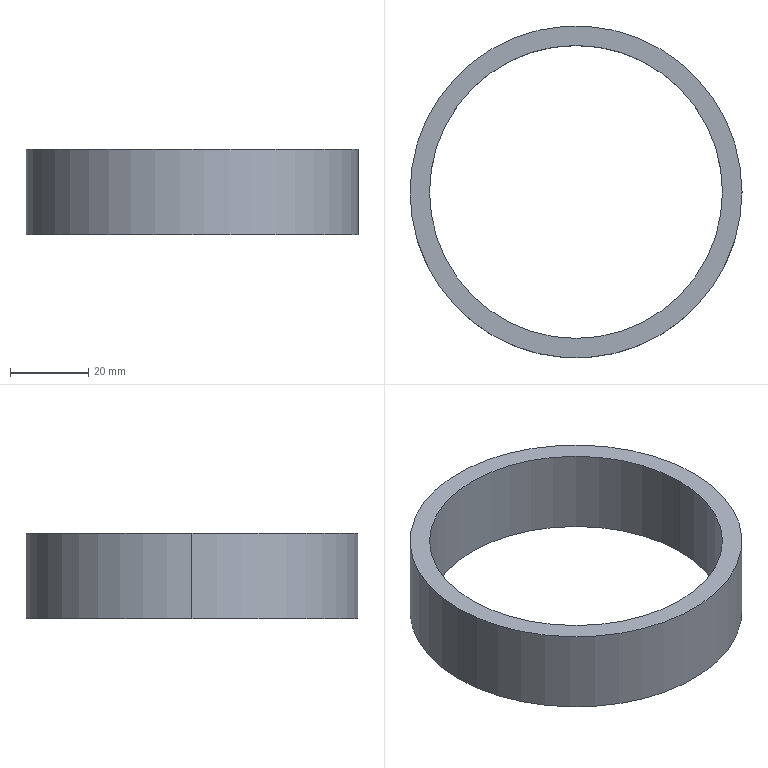Part | SolidWorks | features Extrusion 1 | 1 solid | 6 faces | box 85 x 85 x 22 mm | volume 27646 mm3 | cylinder 4 | plane 2 | commonest cylinder face diameters 75 x2 85 x2
STEP:
#1=CARTESIAN_POINT('',(-37.5,0.,22.));
#2=VERTEX_POINT('',#1);
#3=CARTESIAN_POINT('',(37.5,0.,22.));
#4=VERTEX_POINT('',#3);
#5=CARTESIAN_POINT('',(0.,0.,22.));
#6=DIRECTION('',(0.,0.,1.));
#7=DIRECTION('',(1.,0.,0.));
#8=AXIS2_PLACEMENT_3D('',#5,#6,#7);
#9=CIRCLE('',#8,37.5);
#10=EDGE_CURVE('',#2,#4,#9,.T.);
#11=ORIENTED_EDGE('',*,*,#10,.T.);
#12=CARTESIAN_POINT('',(37.5,0.,0.));
#13=VERTEX_POINT('',#12);
#14=CARTESIAN_POINT('',(37.5,0.,22.));
#15=DIRECTION('',(0.,0.,-1.));
#16=VECTOR('',#15,1000.);
#17=LINE('',#14,#16);
#18=EDGE_CURVE('',#4,#13,#17,.T.);
#19=ORIENTED_EDGE('',*,*,#18,.T.);
#20=CARTESIAN_POINT('',(-37.5,0.,0.));
#21=VERTEX_POINT('',#20);
#22=CARTESIAN_POINT('',(0.,0.,0.));
#23=DIRECTION('',(0.,0.,1.));
#24=DIRECTION('',(1.,0.,0.));
#25=AXIS2_PLACEMENT_3D('',#22,#23,#24);
#26=CIRCLE('',#25,37.5);
#27=EDGE_CURVE('',#21,#13,#26,.T.);
#28=ORIENTED_EDGE('',*,*,#27,.F.);
#29=CARTESIAN_POINT('',(-37.5,0.,22.));
#30=DIRECTION('',(0.,0.,-1.));
#31=VECTOR('',#30,1000.);
#32=LINE('',#29,#31);
#33=EDGE_CURVE('',#2,#21,#32,.T.);
#34=ORIENTED_EDGE('',*,*,#33,.F.);
#35=EDGE_LOOP('',(#11,#19,#28,#34));
#36=FACE_OUTER_BOUND('',#35,.T.);
#37=CARTESIAN_POINT('',(0.,0.,22.));
#38=DIRECTION('',(0.,0.,-1.));
#39=DIRECTION('',(-1.,0.,0.));
#40=AXIS2_PLACEMENT_3D('',#37,#38,#39);
#41=CYLINDRICAL_SURFACE('',#40,37.5);
#42=ADVANCED_FACE('',(#36),#41,.F.);
#43=CARTESIAN_POINT('',(42.5,0.,22.));
#44=VERTEX_POINT('',#43);
#45=CARTESIAN_POINT('',(-42.5,0.,22.));
#46=VERTEX_POINT('',#45);
#47=CARTESIAN_POINT('',(0.,0.,22.));
#48=DIRECTION('',(0.,0.,1.));
#49=DIRECTION('',(1.,0.,0.));
#50=AXIS2_PLACEMENT_3D('',#47,#48,#49);
#51=CIRCLE('',#50,42.5);
#52=EDGE_CURVE('',#44,#46,#51,.T.);
#53=ORIENTED_EDGE('',*,*,#52,.F.);
#54=CARTESIAN_POINT('',(42.5,0.,0.));
#55=VERTEX_POINT('',#54);
#56=CARTESIAN_POINT('',(42.5,0.,22.));
#57=DIRECTION('',(0.,0.,-1.));
#58=VECTOR('',#57,1000.);
#59=LINE('',#56,#58);
#60=EDGE_CURVE('',#44,#55,#59,.T.);
#61=ORIENTED_EDGE('',*,*,#60,.T.);
#62=CARTESIAN_POINT('',(-42.5,0.,0.));
#63=VERTEX_POINT('',#62);
#64=CARTESIAN_POINT('',(0.,0.,0.));
#65=DIRECTION('',(0.,0.,1.));
#66=DIRECTION('',(1.,0.,0.));
#67=AXIS2_PLACEMENT_3D('',#64,#65,#66);
#68=CIRCLE('',#67,42.5);
#69=EDGE_CURVE('',#55,#63,#68,.T.);
#70=ORIENTED_EDGE('',*,*,#69,.T.);
#71=CARTESIAN_POINT('',(-42.5,0.,22.));
#72=DIRECTION('',(0.,0.,-1.));
#73=VECTOR('',#72,1000.);
#74=LINE('',#71,#73);
#75=EDGE_CURVE('',#46,#63,#74,.T.);
#76=ORIENTED_EDGE('',*,*,#75,.F.);
#77=EDGE_LOOP('',(#53,#61,#70,#76));
#78=FACE_OUTER_BOUND('',#77,.T.);
#79=CARTESIAN_POINT('',(0.,0.,22.));
#80=DIRECTION('',(0.,0.,-1.));
#81=DIRECTION('',(-1.,0.,0.));
#82=AXIS2_PLACEMENT_3D('',#79,#80,#81);
#83=CYLINDRICAL_SURFACE('',#82,42.5);
#84=ADVANCED_FACE('',(#78),#83,.T.);
#85=CARTESIAN_POINT('',(0.,0.,22.));
#86=DIRECTION('',(0.,0.,1.));
#87=DIRECTION('',(1.,0.,0.));
#88=AXIS2_PLACEMENT_3D('',#85,#86,#87);
#89=CIRCLE('',#88,42.5);
#90=EDGE_CURVE('',#46,#44,#89,.T.);
#91=ORIENTED_EDGE('',*,*,#90,.T.);
#92=ORIENTED_EDGE('',*,*,#52,.T.);
#93=EDGE_LOOP('',(#91,#92));
#94=FACE_OUTER_BOUND('',#93,.T.);
#95=ORIENTED_EDGE('',*,*,#10,.F.);
#96=CARTESIAN_POINT('',(0.,0.,22.));
#97=DIRECTION('',(0.,0.,1.));
#98=DIRECTION('',(1.,0.,0.));
#99=AXIS2_PLACEMENT_3D('',#96,#97,#98);
#100=CIRCLE('',#99,37.5);
#101=EDGE_CURVE('',#4,#2,#100,.T.);
#102=ORIENTED_EDGE('',*,*,#101,.F.);
#103=EDGE_LOOP('',(#95,#102));
#104=FACE_BOUND('',#103,.T.);
#105=CARTESIAN_POINT('',(0.,0.,22.));
#106=DIRECTION('',(0.,0.,1.));
#107=DIRECTION('',(1.,0.,0.));
#108=AXIS2_PLACEMENT_3D('',#105,#106,#107);
#109=PLANE('',#108);
#110=ADVANCED_FACE('',(#94,#104),#109,.T.);
#111=CARTESIAN_POINT('',(0.,0.,0.));
#112=DIRECTION('',(0.,0.,1.));
#113=DIRECTION('',(1.,0.,0.));
#114=AXIS2_PLACEMENT_3D('',#111,#112,#113);
#115=CIRCLE('',#114,42.5);
#116=EDGE_CURVE('',#63,#55,#115,.T.);
#117=ORIENTED_EDGE('',*,*,#116,.F.);
#118=ORIENTED_EDGE('',*,*,#69,.F.);
#119=EDGE_LOOP('',(#117,#118));
#120=FACE_OUTER_BOUND('',#119,.T.);
#121=ORIENTED_EDGE('',*,*,#27,.T.);
#122=CARTESIAN_POINT('',(0.,0.,0.));
#123=DIRECTION('',(0.,0.,1.));
#124=DIRECTION('',(1.,0.,0.));
#125=AXIS2_PLACEMENT_3D('',#122,#123,#124);
#126=CIRCLE('',#125,37.5);
#127=EDGE_CURVE('',#13,#21,#126,.T.);
#128=ORIENTED_EDGE('',*,*,#127,.T.);
#129=EDGE_LOOP('',(#121,#128));
#130=FACE_BOUND('',#129,.T.);
#131=CARTESIAN_POINT('',(0.,0.,0.));
#132=DIRECTION('',(0.,0.,1.));
#133=DIRECTION('',(1.,0.,0.));
#134=AXIS2_PLACEMENT_3D('',#131,#132,#133);
#135=PLANE('',#134);
#136=ADVANCED_FACE('',(#120,#130),#135,.F.);
#137=ORIENTED_EDGE('',*,*,#60,.F.);
#138=ORIENTED_EDGE('',*,*,#90,.F.);
#139=ORIENTED_EDGE('',*,*,#75,.T.);
#140=ORIENTED_EDGE('',*,*,#116,.T.);
#141=EDGE_LOOP('',(#137,#138,#139,#140));
#142=FACE_OUTER_BOUND('',#141,.T.);
#143=CARTESIAN_POINT('',(0.,0.,22.));
#144=DIRECTION('',(0.,0.,-1.));
#145=DIRECTION('',(-1.,0.,0.));
#146=AXIS2_PLACEMENT_3D('',#143,#144,#145);
#147=CYLINDRICAL_SURFACE('',#146,42.5);
#148=ADVANCED_FACE('',(#142),#147,.T.);
#149=ORIENTED_EDGE('',*,*,#18,.F.);
#150=ORIENTED_EDGE('',*,*,#101,.T.);
#151=ORIENTED_EDGE('',*,*,#33,.T.);
#152=ORIENTED_EDGE('',*,*,#127,.F.);
#153=EDGE_LOOP('',(#149,#150,#151,#152));
#154=FACE_OUTER_BOUND('',#153,.T.);
#155=CARTESIAN_POINT('',(0.,0.,22.));
#156=DIRECTION('',(0.,0.,-1.));
#157=DIRECTION('',(-1.,0.,0.));
#158=AXIS2_PLACEMENT_3D('',#155,#156,#157);
#159=CYLINDRICAL_SURFACE('',#158,37.5);
#160=ADVANCED_FACE('',(#154),#159,.F.);
#161=CLOSED_SHELL('',(#42,#84,#110,#136,#148,#160));
#162=MANIFOLD_SOLID_BREP('',#161);
#163=CARTESIAN_POINT('',(0.,0.,0.));
#164=DIRECTION('',(0.,0.,1.));
#165=DIRECTION('',(1.,0.,0.));
#166=AXIS2_PLACEMENT_3D('',#163,#164,#165);
#167=(LENGTH_UNIT()NAMED_UNIT(*)SI_UNIT(.MILLI.,.METRE.));
#168=UNCERTAINTY_MEASURE_WITH_UNIT(LENGTH_MEASURE(0.00001),#167,'','');
#169=(NAMED_UNIT(*)PLANE_ANGLE_UNIT()SI_UNIT($,.RADIAN.));
#170=(NAMED_UNIT(*)SI_UNIT($,.STERADIAN.)SOLID_ANGLE_UNIT());
#171=(GEOMETRIC_REPRESENTATION_CONTEXT(3)GLOBAL_UNCERTAINTY_ASSIGNED_CONTEXT((#168))GLOBAL_UNIT_ASSIGNED_CONTEXT((#167,#169,#170))REPRESENTATION_CONTEXT('',''));
#172=ADVANCED_BREP_SHAPE_REPRESENTATION('',(#162,#166),#171);